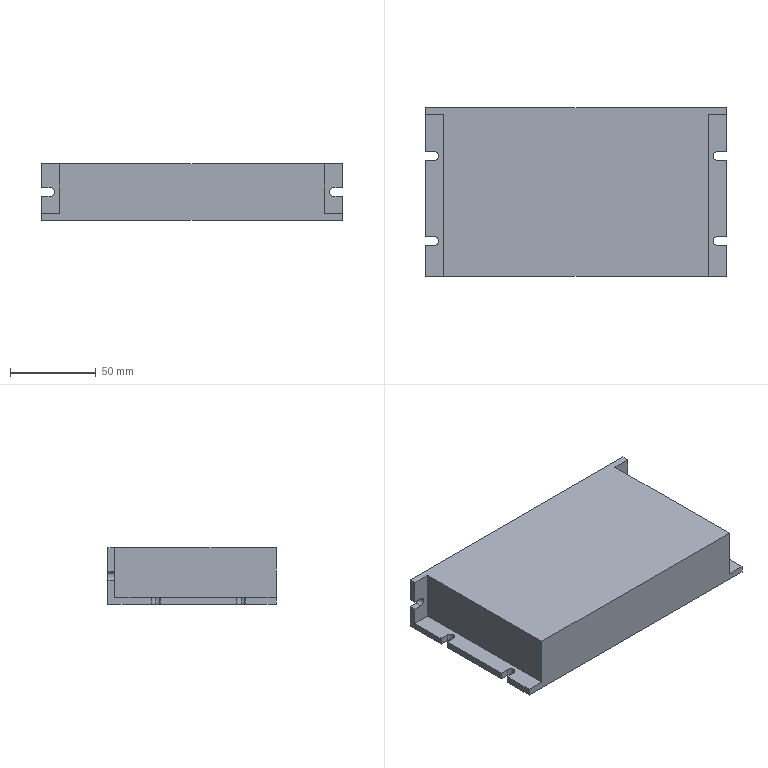Part | SolidWorks | features BaseBody 1 | 1 solid | 38 faces | box 175 x 98 x 33 mm | volume 507848 mm3 | plane 30 | cylinder 8 | commonest cylinder face diameters 5 x8
STEP:
#1=CARTESIAN_POINT('',(82.5,49.,14.));
#2=VERTEX_POINT('',#1);
#3=CARTESIAN_POINT('',(87.5,49.,14.));
#4=VERTEX_POINT('',#3);
#5=CARTESIAN_POINT('',(-87.5,49.,14.));
#6=DIRECTION('',(1.,0.,0.));
#7=VECTOR('',#6,1000.);
#8=LINE('',#5,#7);
#9=EDGE_CURVE('',#2,#4,#8,.T.);
#10=ORIENTED_EDGE('',*,*,#9,.F.);
#11=CARTESIAN_POINT('',(82.5,45.,14.));
#12=VERTEX_POINT('',#11);
#13=CARTESIAN_POINT('',(82.5,139.,14.));
#14=DIRECTION('',(0.,-1.,0.));
#15=VECTOR('',#14,1000.);
#16=LINE('',#13,#15);
#17=EDGE_CURVE('',#2,#12,#16,.T.);
#18=ORIENTED_EDGE('',*,*,#17,.T.);
#19=CARTESIAN_POINT('',(87.5,45.,14.));
#20=VERTEX_POINT('',#19);
#21=CARTESIAN_POINT('',(82.5,45.,14.));
#22=DIRECTION('',(1.,0.,0.));
#23=VECTOR('',#22,1000.);
#24=LINE('',#21,#23);
#25=EDGE_CURVE('',#12,#20,#24,.T.);
#26=ORIENTED_EDGE('',*,*,#25,.T.);
#27=CARTESIAN_POINT('',(87.5,-49.,14.));
#28=DIRECTION('',(0.,-1.,0.));
#29=VECTOR('',#28,1000.);
#30=LINE('',#27,#29);
#31=EDGE_CURVE('',#4,#20,#30,.T.);
#32=ORIENTED_EDGE('',*,*,#31,.F.);
#33=EDGE_LOOP('',(#10,#18,#26,#32));
#34=FACE_OUTER_BOUND('',#33,.T.);
#35=CARTESIAN_POINT('',(82.5,139.,14.));
#36=DIRECTION('',(0.,0.,-1.));
#37=DIRECTION('',(0.,-1.,0.));
#38=AXIS2_PLACEMENT_3D('',#35,#36,#37);
#39=PLANE('',#38);
#40=ADVANCED_FACE('',(#34),#39,.F.);
#41=CARTESIAN_POINT('',(82.5,45.,19.));
#42=VERTEX_POINT('',#41);
#43=CARTESIAN_POINT('',(87.5,45.,19.));
#44=VERTEX_POINT('',#43);
#45=CARTESIAN_POINT('',(0.,45.,19.));
#46=DIRECTION('',(1.,0.,0.));
#47=VECTOR('',#46,1000.);
#48=LINE('',#45,#47);
#49=EDGE_CURVE('',#42,#44,#48,.T.);
#50=ORIENTED_EDGE('',*,*,#49,.F.);
#51=CARTESIAN_POINT('',(82.5,49.,19.));
#52=VERTEX_POINT('',#51);
#53=CARTESIAN_POINT('',(82.5,139.,19.));
#54=DIRECTION('',(0.,-1.,0.));
#55=VECTOR('',#54,1000.);
#56=LINE('',#53,#55);
#57=EDGE_CURVE('',#52,#42,#56,.T.);
#58=ORIENTED_EDGE('',*,*,#57,.F.);
#59=CARTESIAN_POINT('',(87.5,49.,19.));
#60=VERTEX_POINT('',#59);
#61=CARTESIAN_POINT('',(-87.5,49.,19.));
#62=DIRECTION('',(-1.,0.,0.));
#63=VECTOR('',#62,1000.);
#64=LINE('',#61,#63);
#65=EDGE_CURVE('',#60,#52,#64,.T.);
#66=ORIENTED_EDGE('',*,*,#65,.F.);
#67=CARTESIAN_POINT('',(87.5,-49.,19.));
#68=DIRECTION('',(0.,1.,0.));
#69=VECTOR('',#68,1000.);
#70=LINE('',#67,#69);
#71=EDGE_CURVE('',#44,#60,#70,.T.);
#72=ORIENTED_EDGE('',*,*,#71,.F.);
#73=EDGE_LOOP('',(#50,#58,#66,#72));
#74=FACE_OUTER_BOUND('',#73,.T.);
#75=CARTESIAN_POINT('',(92.4,139.,19.));
#76=DIRECTION('',(0.,0.,1.));
#77=DIRECTION('',(1.,0.,0.));
#78=AXIS2_PLACEMENT_3D('',#75,#76,#77);
#79=PLANE('',#78);
#80=ADVANCED_FACE('',(#74),#79,.F.);
#81=ORIENTED_EDGE('',*,*,#57,.T.);
#82=CARTESIAN_POINT('',(82.5,45.,16.5));
#83=DIRECTION('',(0.,-1.,0.));
#84=DIRECTION('',(0.,0.,1.));
#85=AXIS2_PLACEMENT_3D('',#82,#83,#84);
#86=CIRCLE('',#85,2.5);
#87=EDGE_CURVE('',#42,#12,#86,.T.);
#88=ORIENTED_EDGE('',*,*,#87,.T.);
#89=ORIENTED_EDGE('',*,*,#17,.F.);
#90=CARTESIAN_POINT('',(82.5,49.,16.5));
#91=DIRECTION('',(0.,-1.,0.));
#92=DIRECTION('',(0.,0.,-1.));
#93=AXIS2_PLACEMENT_3D('',#90,#91,#92);
#94=CIRCLE('',#93,2.5);
#95=EDGE_CURVE('',#52,#2,#94,.T.);
#96=ORIENTED_EDGE('',*,*,#95,.F.);
#97=EDGE_LOOP('',(#81,#88,#89,#96));
#98=FACE_OUTER_BOUND('',#97,.T.);
#99=CARTESIAN_POINT('',(82.5,139.,16.5));
#100=DIRECTION('',(0.,-1.,0.));
#101=DIRECTION('',(0.,0.,-1.));
#102=AXIS2_PLACEMENT_3D('',#99,#100,#101);
#103=CYLINDRICAL_SURFACE('',#102,2.5);
#104=ADVANCED_FACE('',(#98),#103,.F.);
#105=CARTESIAN_POINT('',(-82.5,49.,19.));
#106=VERTEX_POINT('',#105);
#107=CARTESIAN_POINT('',(-82.5,45.,19.));
#108=VERTEX_POINT('',#107);
#109=CARTESIAN_POINT('',(-82.5,139.,19.));
#110=DIRECTION('',(0.,-1.,0.));
#111=VECTOR('',#110,1000.);
#112=LINE('',#109,#111);
#113=EDGE_CURVE('',#106,#108,#112,.T.);
#114=ORIENTED_EDGE('',*,*,#113,.T.);
#115=CARTESIAN_POINT('',(-87.5,45.,19.));
#116=VERTEX_POINT('',#115);
#117=CARTESIAN_POINT('',(-92.4,45.,19.));
#118=DIRECTION('',(-1.,0.,0.));
#119=VECTOR('',#118,1000.);
#120=LINE('',#117,#119);
#121=EDGE_CURVE('',#108,#116,#120,.T.);
#122=ORIENTED_EDGE('',*,*,#121,.T.);
#123=CARTESIAN_POINT('',(-87.5,49.,19.));
#124=VERTEX_POINT('',#123);
#125=CARTESIAN_POINT('',(-87.5,-49.,19.));
#126=DIRECTION('',(0.,-1.,0.));
#127=VECTOR('',#126,1000.);
#128=LINE('',#125,#127);
#129=EDGE_CURVE('',#124,#116,#128,.T.);
#130=ORIENTED_EDGE('',*,*,#129,.F.);
#131=CARTESIAN_POINT('',(-87.5,49.,19.));
#132=DIRECTION('',(-1.,0.,0.));
#133=VECTOR('',#132,1000.);
#134=LINE('',#131,#133);
#135=EDGE_CURVE('',#106,#124,#134,.T.);
#136=ORIENTED_EDGE('',*,*,#135,.F.);
#137=EDGE_LOOP('',(#114,#122,#130,#136));
#138=FACE_OUTER_BOUND('',#137,.T.);
#139=CARTESIAN_POINT('',(-92.4,139.,19.));
#140=DIRECTION('',(0.,0.,1.));
#141=DIRECTION('',(1.,0.,0.));
#142=AXIS2_PLACEMENT_3D('',#139,#140,#141);
#143=PLANE('',#142);
#144=ADVANCED_FACE('',(#138),#143,.F.);
#145=CARTESIAN_POINT('',(-87.5,45.,14.));
#146=VERTEX_POINT('',#145);
#147=CARTESIAN_POINT('',(-87.5,49.,14.));
#148=VERTEX_POINT('',#147);
#149=CARTESIAN_POINT('',(-87.5,-49.,14.));
#150=DIRECTION('',(0.,1.,0.));
#151=VECTOR('',#150,1000.);
#152=LINE('',#149,#151);
#153=EDGE_CURVE('',#146,#148,#152,.T.);
#154=ORIENTED_EDGE('',*,*,#153,.F.);
#155=CARTESIAN_POINT('',(-82.5,45.,14.));
#156=VERTEX_POINT('',#155);
#157=CARTESIAN_POINT('',(0.,45.,14.));
#158=DIRECTION('',(1.,0.,0.));
#159=VECTOR('',#158,1000.);
#160=LINE('',#157,#159);
#161=EDGE_CURVE('',#146,#156,#160,.T.);
#162=ORIENTED_EDGE('',*,*,#161,.T.);
#163=CARTESIAN_POINT('',(-82.5,49.,14.));
#164=VERTEX_POINT('',#163);
#165=CARTESIAN_POINT('',(-82.5,139.,14.));
#166=DIRECTION('',(0.,-1.,0.));
#167=VECTOR('',#166,1000.);
#168=LINE('',#165,#167);
#169=EDGE_CURVE('',#164,#156,#168,.T.);
#170=ORIENTED_EDGE('',*,*,#169,.F.);
#171=CARTESIAN_POINT('',(-87.5,49.,14.));
#172=DIRECTION('',(1.,0.,0.));
#173=VECTOR('',#172,1000.);
#174=LINE('',#171,#173);
#175=EDGE_CURVE('',#148,#164,#174,.T.);
#176=ORIENTED_EDGE('',*,*,#175,.F.);
#177=EDGE_LOOP('',(#154,#162,#170,#176));
#178=FACE_OUTER_BOUND('',#177,.T.);
#179=CARTESIAN_POINT('',(-82.5,139.,14.));
#180=DIRECTION('',(0.,0.,-1.));
#181=DIRECTION('',(0.,-1.,0.));
#182=AXIS2_PLACEMENT_3D('',#179,#180,#181);
#183=PLANE('',#182);
#184=ADVANCED_FACE('',(#178),#183,.F.);
#185=ORIENTED_EDGE('',*,*,#169,.T.);
#186=CARTESIAN_POINT('',(-82.5,45.,16.5));
#187=DIRECTION('',(0.,-1.,0.));
#188=DIRECTION('',(0.,0.,-1.));
#189=AXIS2_PLACEMENT_3D('',#186,#187,#188);
#190=CIRCLE('',#189,2.5);
#191=EDGE_CURVE('',#156,#108,#190,.T.);
#192=ORIENTED_EDGE('',*,*,#191,.T.);
#193=ORIENTED_EDGE('',*,*,#113,.F.);
#194=CARTESIAN_POINT('',(-82.5,49.,16.5));
#195=DIRECTION('',(0.,-1.,0.));
#196=DIRECTION('',(0.,0.,-1.));
#197=AXIS2_PLACEMENT_3D('',#194,#195,#196);
#198=CIRCLE('',#197,2.5);
#199=EDGE_CURVE('',#164,#106,#198,.T.);
#200=ORIENTED_EDGE('',*,*,#199,.F.);
#201=EDGE_LOOP('',(#185,#192,#193,#200));
#202=FACE_OUTER_BOUND('',#201,.T.);
#203=CARTESIAN_POINT('',(-82.5,139.,16.5));
#204=DIRECTION('',(0.,-1.,0.));
#205=DIRECTION('',(0.,0.,-1.));
#206=AXIS2_PLACEMENT_3D('',#203,#204,#205);
#207=CYLINDRICAL_SURFACE('',#206,2.5);
#208=ADVANCED_FACE('',(#202),#207,.F.);
#209=CARTESIAN_POINT('',(82.25,18.5,0.));
#210=VERTEX_POINT('',#209);
#211=CARTESIAN_POINT('',(82.25,23.5,0.));
#212=VERTEX_POINT('',#211);
#213=CARTESIAN_POINT('',(82.25,21.,0.));
#214=DIRECTION('',(0.,0.,-1.));
#215=DIRECTION('',(-1.,0.,0.));
#216=AXIS2_PLACEMENT_3D('',#213,#214,#215);
#217=CIRCLE('',#216,2.5);
#218=EDGE_CURVE('',#210,#212,#217,.T.);
#219=ORIENTED_EDGE('',*,*,#218,.T.);
#220=CARTESIAN_POINT('',(82.25,23.5,4.));
#221=VERTEX_POINT('',#220);
#222=CARTESIAN_POINT('',(82.25,23.5,-90.));
#223=DIRECTION('',(0.,0.,1.));
#224=VECTOR('',#223,1000.);
#225=LINE('',#222,#224);
#226=EDGE_CURVE('',#212,#221,#225,.T.);
#227=ORIENTED_EDGE('',*,*,#226,.T.);
#228=CARTESIAN_POINT('',(82.25,18.5,4.));
#229=VERTEX_POINT('',#228);
#230=CARTESIAN_POINT('',(82.25,21.,4.));
#231=DIRECTION('',(0.,0.,1.));
#232=DIRECTION('',(-1.,0.,0.));
#233=AXIS2_PLACEMENT_3D('',#230,#231,#232);
#234=CIRCLE('',#233,2.5);
#235=EDGE_CURVE('',#221,#229,#234,.T.);
#236=ORIENTED_EDGE('',*,*,#235,.T.);
#237=CARTESIAN_POINT('',(82.25,18.5,-90.));
#238=DIRECTION('',(0.,0.,1.));
#239=VECTOR('',#238,1000.);
#240=LINE('',#237,#239);
#241=EDGE_CURVE('',#210,#229,#240,.T.);
#242=ORIENTED_EDGE('',*,*,#241,.F.);
#243=EDGE_LOOP('',(#219,#227,#236,#242));
#244=FACE_OUTER_BOUND('',#243,.T.);
#245=CARTESIAN_POINT('',(82.25,21.,-90.));
#246=DIRECTION('',(0.,0.,1.));
#247=DIRECTION('',(1.,0.,0.));
#248=AXIS2_PLACEMENT_3D('',#245,#246,#247);
#249=CYLINDRICAL_SURFACE('',#248,2.5);
#250=ADVANCED_FACE('',(#244),#249,.F.);
#251=CARTESIAN_POINT('',(87.5,18.5,0.));
#252=VERTEX_POINT('',#251);
#253=CARTESIAN_POINT('',(0.,18.5,0.));
#254=DIRECTION('',(-1.,0.,0.));
#255=VECTOR('',#254,1000.);
#256=LINE('',#253,#255);
#257=EDGE_CURVE('',#252,#210,#256,.T.);
#258=ORIENTED_EDGE('',*,*,#257,.T.);
#259=ORIENTED_EDGE('',*,*,#241,.T.);
#260=CARTESIAN_POINT('',(87.5,18.5,4.));
#261=VERTEX_POINT('',#260);
#262=CARTESIAN_POINT('',(101.009,18.5,4.));
#263=DIRECTION('',(1.,0.,0.));
#264=VECTOR('',#263,1000.);
#265=LINE('',#262,#264);
#266=EDGE_CURVE('',#229,#261,#265,.T.);
#267=ORIENTED_EDGE('',*,*,#266,.T.);
#268=CARTESIAN_POINT('',(87.5,18.5,33.));
#269=DIRECTION('',(0.,0.,1.));
#270=VECTOR('',#269,1000.);
#271=LINE('',#268,#270);
#272=EDGE_CURVE('',#252,#261,#271,.T.);
#273=ORIENTED_EDGE('',*,*,#272,.F.);
#274=EDGE_LOOP('',(#258,#259,#267,#273));
#275=FACE_OUTER_BOUND('',#274,.T.);
#276=CARTESIAN_POINT('',(101.009,18.5,-90.));
#277=DIRECTION('',(0.,-1.,0.));
#278=DIRECTION('',(0.,0.,-1.));
#279=AXIS2_PLACEMENT_3D('',#276,#277,#278);
#280=PLANE('',#279);
#281=ADVANCED_FACE('',(#275),#280,.F.);
#282=CARTESIAN_POINT('',(87.5,23.5,4.));
#283=VERTEX_POINT('',#282);
#284=CARTESIAN_POINT('',(87.5,23.5,4.));
#285=DIRECTION('',(1.,0.,0.));
#286=VECTOR('',#285,1000.);
#287=LINE('',#284,#286);
#288=EDGE_CURVE('',#221,#283,#287,.T.);
#289=ORIENTED_EDGE('',*,*,#288,.F.);
#290=ORIENTED_EDGE('',*,*,#226,.F.);
#291=CARTESIAN_POINT('',(87.5,23.5,0.));
#292=VERTEX_POINT('',#291);
#293=CARTESIAN_POINT('',(0.,23.5,0.));
#294=DIRECTION('',(1.,0.,0.));
#295=VECTOR('',#294,1000.);
#296=LINE('',#293,#295);
#297=EDGE_CURVE('',#212,#292,#296,.T.);
#298=ORIENTED_EDGE('',*,*,#297,.T.);
#299=CARTESIAN_POINT('',(87.5,23.5,33.));
#300=DIRECTION('',(0.,0.,-1.));
#301=VECTOR('',#300,1000.);
#302=LINE('',#299,#301);
#303=EDGE_CURVE('',#283,#292,#302,.T.);
#304=ORIENTED_EDGE('',*,*,#303,.F.);
#305=EDGE_LOOP('',(#289,#290,#298,#304));
#306=FACE_OUTER_BOUND('',#305,.T.);
#307=CARTESIAN_POINT('',(82.25,23.5,-90.));
#308=DIRECTION('',(0.,1.,0.));
#309=DIRECTION('',(1.,0.,0.));
#310=AXIS2_PLACEMENT_3D('',#307,#308,#309);
#311=PLANE('',#310);
#312=ADVANCED_FACE('',(#306),#311,.F.);
#313=CARTESIAN_POINT('',(82.25,-31.,0.));
#314=VERTEX_POINT('',#313);
#315=CARTESIAN_POINT('',(82.25,-26.,0.));
#316=VERTEX_POINT('',#315);
#317=CARTESIAN_POINT('',(82.25,-28.5,0.));
#318=DIRECTION('',(0.,0.,-1.));
#319=DIRECTION('',(-1.,0.,0.));
#320=AXIS2_PLACEMENT_3D('',#317,#318,#319);
#321=CIRCLE('',#320,2.5);
#322=EDGE_CURVE('',#314,#316,#321,.T.);
#323=ORIENTED_EDGE('',*,*,#322,.T.);
#324=CARTESIAN_POINT('',(82.25,-26.,4.));
#325=VERTEX_POINT('',#324);
#326=CARTESIAN_POINT('',(82.25,-26.,-90.));
#327=DIRECTION('',(0.,0.,1.));
#328=VECTOR('',#327,1000.);
#329=LINE('',#326,#328);
#330=EDGE_CURVE('',#316,#325,#329,.T.);
#331=ORIENTED_EDGE('',*,*,#330,.T.);
#332=CARTESIAN_POINT('',(82.25,-31.,4.));
#333=VERTEX_POINT('',#332);
#334=CARTESIAN_POINT('',(82.25,-28.5,4.));
#335=DIRECTION('',(0.,0.,1.));
#336=DIRECTION('',(-1.,0.,0.));
#337=AXIS2_PLACEMENT_3D('',#334,#335,#336);
#338=CIRCLE('',#337,2.5);
#339=EDGE_CURVE('',#325,#333,#338,.T.);
#340=ORIENTED_EDGE('',*,*,#339,.T.);
#341=CARTESIAN_POINT('',(82.25,-31.,-90.));
#342=DIRECTION('',(0.,0.,1.));
#343=VECTOR('',#342,1000.);
#344=LINE('',#341,#343);
#345=EDGE_CURVE('',#314,#333,#344,.T.);
#346=ORIENTED_EDGE('',*,*,#345,.F.);
#347=EDGE_LOOP('',(#323,#331,#340,#346));
#348=FACE_OUTER_BOUND('',#347,.T.);
#349=CARTESIAN_POINT('',(82.25,-28.5,-90.));
#350=DIRECTION('',(0.,0.,1.));
#351=DIRECTION('',(1.,0.,0.));
#352=AXIS2_PLACEMENT_3D('',#349,#350,#351);
#353=CYLINDRICAL_SURFACE('',#352,2.5);
#354=ADVANCED_FACE('',(#348),#353,.F.);
#355=CARTESIAN_POINT('',(87.5,-31.,0.));
#356=VERTEX_POINT('',#355);
#357=CARTESIAN_POINT('',(0.,-31.,0.));
#358=DIRECTION('',(-1.,0.,0.));
#359=VECTOR('',#358,1000.);
#360=LINE('',#357,#359);
#361=EDGE_CURVE('',#356,#314,#360,.T.);
#362=ORIENTED_EDGE('',*,*,#361,.T.);
#363=ORIENTED_EDGE('',*,*,#345,.T.);
#364=CARTESIAN_POINT('',(87.5,-31.,4.));
#365=VERTEX_POINT('',#364);
#366=CARTESIAN_POINT('',(82.25,-31.,4.));
#367=DIRECTION('',(1.,0.,0.));
#368=VECTOR('',#367,1000.);
#369=LINE('',#366,#368);
#370=EDGE_CURVE('',#333,#365,#369,.T.);
#371=ORIENTED_EDGE('',*,*,#370,.T.);
#372=CARTESIAN_POINT('',(87.5,-31.,33.));
#373=DIRECTION('',(0.,0.,1.));
#374=VECTOR('',#373,1000.);
#375=LINE('',#372,#374);
#376=EDGE_CURVE('',#356,#365,#375,.T.);
#377=ORIENTED_EDGE('',*,*,#376,.F.);
#378=EDGE_LOOP('',(#362,#363,#371,#377));
#379=FACE_OUTER_BOUND('',#378,.T.);
#380=CARTESIAN_POINT('',(82.25,-31.,-90.));
#381=DIRECTION('',(0.,-1.,0.));
#382=DIRECTION('',(0.,0.,-1.));
#383=AXIS2_PLACEMENT_3D('',#380,#381,#382);
#384=PLANE('',#383);
#385=ADVANCED_FACE('',(#379),#384,.F.);
#386=CARTESIAN_POINT('',(87.5,-26.,4.));
#387=VERTEX_POINT('',#386);
#388=CARTESIAN_POINT('',(87.5,-26.,4.));
#389=DIRECTION('',(1.,0.,0.));
#390=VECTOR('',#389,1000.);
#391=LINE('',#388,#390);
#392=EDGE_CURVE('',#325,#387,#391,.T.);
#393=ORIENTED_EDGE('',*,*,#392,.F.);
#394=ORIENTED_EDGE('',*,*,#330,.F.);
#395=CARTESIAN_POINT('',(87.5,-26.,0.));
#396=VERTEX_POINT('',#395);
#397=CARTESIAN_POINT('',(0.,-26.,0.));
#398=DIRECTION('',(1.,0.,0.));
#399=VECTOR('',#398,1000.);
#400=LINE('',#397,#399);
#401=EDGE_CURVE('',#316,#396,#400,.T.);
#402=ORIENTED_EDGE('',*,*,#401,.T.);
#403=CARTESIAN_POINT('',(87.5,-26.,33.));
#404=DIRECTION('',(0.,0.,-1.));
#405=VECTOR('',#404,1000.);
#406=LINE('',#403,#405);
#407=EDGE_CURVE('',#387,#396,#406,.T.);
#408=ORIENTED_EDGE('',*,*,#407,.F.);
#409=EDGE_LOOP('',(#393,#394,#402,#408));
#410=FACE_OUTER_BOUND('',#409,.T.);
#411=CARTESIAN_POINT('',(101.009,-26.,-90.));
#412=DIRECTION('',(0.,1.,0.));
#413=DIRECTION('',(1.,0.,0.));
#414=AXIS2_PLACEMENT_3D('',#411,#412,#413);
#415=PLANE('',#414);
#416=ADVANCED_FACE('',(#410),#415,.F.);
#417=CARTESIAN_POINT('',(-79.75,-28.5,0.));
#418=VERTEX_POINT('',#417);
#419=CARTESIAN_POINT('',(-79.75,-28.5,4.));
#420=VERTEX_POINT('',#419);
#421=CARTESIAN_POINT('',(-79.75,-28.5,-90.));
#422=DIRECTION('',(0.,0.,1.));
#423=VECTOR('',#422,1000.);
#424=LINE('',#421,#423);
#425=EDGE_CURVE('',#418,#420,#424,.T.);
#426=ORIENTED_EDGE('',*,*,#425,.F.);
#427=CARTESIAN_POINT('',(-82.25,-31.,0.));
#428=VERTEX_POINT('',#427);
#429=CARTESIAN_POINT('',(-82.25,-28.5,0.));
#430=DIRECTION('',(0.,0.,-1.));
#431=DIRECTION('',(-1.,0.,0.));
#432=AXIS2_PLACEMENT_3D('',#429,#430,#431);
#433=CIRCLE('',#432,2.5);
#434=EDGE_CURVE('',#418,#428,#433,.T.);
#435=ORIENTED_EDGE('',*,*,#434,.T.);
#436=CARTESIAN_POINT('',(-82.25,-31.,4.));
#437=VERTEX_POINT('',#436);
#438=CARTESIAN_POINT('',(-82.25,-31.,-90.));
#439=DIRECTION('',(0.,0.,1.));
#440=VECTOR('',#439,1000.);
#441=LINE('',#438,#440);
#442=EDGE_CURVE('',#428,#437,#441,.T.);
#443=ORIENTED_EDGE('',*,*,#442,.T.);
#444=CARTESIAN_POINT('',(-82.25,-28.5,4.));
#445=DIRECTION('',(0.,0.,1.));
#446=DIRECTION('',(1.,0.,0.));
#447=AXIS2_PLACEMENT_3D('',#444,#445,#446);
#448=CIRCLE('',#447,2.5);
#449=EDGE_CURVE('',#437,#420,#448,.T.);
#450=ORIENTED_EDGE('',*,*,#449,.T.);
#451=EDGE_LOOP('',(#426,#435,#443,#450));
#452=FACE_OUTER_BOUND('',#451,.T.);
#453=CARTESIAN_POINT('',(-82.25,-28.5,-90.));
#454=DIRECTION('',(0.,0.,1.));
#455=DIRECTION('',(1.,0.,0.));
#456=AXIS2_PLACEMENT_3D('',#453,#454,#455);
#457=CYLINDRICAL_SURFACE('',#456,2.5);
#458=ADVANCED_FACE('',(#452),#457,.F.);
#459=CARTESIAN_POINT('',(-87.5,-26.,0.));
#460=VERTEX_POINT('',#459);
#461=CARTESIAN_POINT('',(-82.25,-26.,0.));
#462=VERTEX_POINT('',#461);
#463=CARTESIAN_POINT('',(0.,-26.,0.));
#464=DIRECTION('',(1.,0.,0.));
#465=VECTOR('',#464,1000.);
#466=LINE('',#463,#465);
#467=EDGE_CURVE('',#460,#462,#466,.T.);
#468=ORIENTED_EDGE('',*,*,#467,.T.);
#469=CARTESIAN_POINT('',(-82.25,-26.,4.));
#470=VERTEX_POINT('',#469);
#471=CARTESIAN_POINT('',(-82.25,-26.,-90.));
#472=DIRECTION('',(0.,0.,1.));
#473=VECTOR('',#472,1000.);
#474=LINE('',#471,#473);
#475=EDGE_CURVE('',#462,#470,#474,.T.);
#476=ORIENTED_EDGE('',*,*,#475,.T.);
#477=CARTESIAN_POINT('',(-87.5,-26.,4.));
#478=VERTEX_POINT('',#477);
#479=CARTESIAN_POINT('',(-101.009,-26.,4.));
#480=DIRECTION('',(-1.,0.,0.));
#481=VECTOR('',#480,1000.);
#482=LINE('',#479,#481);
#483=EDGE_CURVE('',#470,#478,#482,.T.);
#484=ORIENTED_EDGE('',*,*,#483,.T.);
#485=CARTESIAN_POINT('',(-87.5,-26.,33.));
#486=DIRECTION('',(0.,0.,1.));
#487=VECTOR('',#486,1000.);
#488=LINE('',#485,#487);
#489=EDGE_CURVE('',#460,#478,#488,.T.);
#490=ORIENTED_EDGE('',*,*,#489,.F.);
#491=EDGE_LOOP('',(#468,#476,#484,#490));
#492=FACE_OUTER_BOUND('',#491,.T.);
#493=CARTESIAN_POINT('',(-101.009,-26.,-90.));
#494=DIRECTION('',(0.,1.,0.));
#495=DIRECTION('',(1.,0.,0.));
#496=AXIS2_PLACEMENT_3D('',#493,#494,#495);
#497=PLANE('',#496);
#498=ADVANCED_FACE('',(#492),#497,.F.);
#499=CARTESIAN_POINT('',(-87.5,-31.,4.));
#500=VERTEX_POINT('',#499);
#501=CARTESIAN_POINT('',(-87.5,-31.,4.));
#502=DIRECTION('',(-1.,0.,0.));
#503=VECTOR('',#502,1000.);
#504=LINE('',#501,#503);
#505=EDGE_CURVE('',#437,#500,#504,.T.);
#506=ORIENTED_EDGE('',*,*,#505,.F.);
#507=ORIENTED_EDGE('',*,*,#442,.F.);
#508=CARTESIAN_POINT('',(-87.5,-31.,0.));
#509=VERTEX_POINT('',#508);
#510=CARTESIAN_POINT('',(0.,-31.,0.));
#511=DIRECTION('',(-1.,0.,0.));
#512=VECTOR('',#511,1000.);
#513=LINE('',#510,#512);
#514=EDGE_CURVE('',#428,#509,#513,.T.);
#515=ORIENTED_EDGE('',*,*,#514,.T.);
#516=CARTESIAN_POINT('',(-87.5,-31.,33.));
#517=DIRECTION('',(0.,0.,-1.));
#518=VECTOR('',#517,1000.);
#519=LINE('',#516,#518);
#520=EDGE_CURVE('',#500,#509,#519,.T.);
#521=ORIENTED_EDGE('',*,*,#520,.F.);
#522=EDGE_LOOP('',(#506,#507,#515,#521));
#523=FACE_OUTER_BOUND('',#522,.T.);
#524=CARTESIAN_POINT('',(-82.25,-31.,-90.));
#525=DIRECTION('',(0.,-1.,0.));
#526=DIRECTION('',(0.,0.,-1.));
#527=AXIS2_PLACEMENT_3D('',#524,#525,#526);
#528=PLANE('',#527);
#529=ADVANCED_FACE('',(#523),#528,.F.);
#530=CARTESIAN_POINT('',(-79.75,21.,0.));
#531=VERTEX_POINT('',#530);
#532=CARTESIAN_POINT('',(-79.75,21.,4.));
#533=VERTEX_POINT('',#532);
#534=CARTESIAN_POINT('',(-79.75,21.,-90.));
#535=DIRECTION('',(0.,0.,1.));
#536=VECTOR('',#535,1000.);
#537=LINE('',#534,#536);
#538=EDGE_CURVE('',#531,#533,#537,.T.);
#539=ORIENTED_EDGE('',*,*,#538,.F.);
#540=CARTESIAN_POINT('',(-82.25,18.5,0.));
#541=VERTEX_POINT('',#540);
#542=CARTESIAN_POINT('',(-82.25,21.,0.));
#543=DIRECTION('',(0.,0.,-1.));
#544=DIRECTION('',(-1.,0.,0.));
#545=AXIS2_PLACEMENT_3D('',#542,#543,#544);
#546=CIRCLE('',#545,2.5);
#547=EDGE_CURVE('',#531,#541,#546,.T.);
#548=ORIENTED_EDGE('',*,*,#547,.T.);
#549=CARTESIAN_POINT('',(-82.25,18.5,4.));
#550=VERTEX_POINT('',#549);
#551=CARTESIAN_POINT('',(-82.25,18.5,-90.));
#552=DIRECTION('',(0.,0.,1.));
#553=VECTOR('',#552,1000.);
#554=LINE('',#551,#553);
#555=EDGE_CURVE('',#541,#550,#554,.T.);
#556=ORIENTED_EDGE('',*,*,#555,.T.);
#557=CARTESIAN_POINT('',(-82.25,21.,4.));
#558=DIRECTION('',(0.,0.,1.));
#559=DIRECTION('',(1.,0.,0.));
#560=AXIS2_PLACEMENT_3D('',#557,#558,#559);
#561=CIRCLE('',#560,2.5);
#562=EDGE_CURVE('',#550,#533,#561,.T.);
#563=ORIENTED_EDGE('',*,*,#562,.T.);
#564=EDGE_LOOP('',(#539,#548,#556,#563));
#565=FACE_OUTER_BOUND('',#564,.T.);
#566=CARTESIAN_POINT('',(-82.25,21.,-90.));
#567=DIRECTION('',(0.,0.,1.));
#568=DIRECTION('',(1.,0.,0.));
#569=AXIS2_PLACEMENT_3D('',#566,#567,#568);
#570=CYLINDRICAL_SURFACE('',#569,2.5);
#571=ADVANCED_FACE('',(#565),#570,.F.);
#572=CARTESIAN_POINT('',(-87.5,23.5,0.));
#573=VERTEX_POINT('',#572);
#574=CARTESIAN_POINT('',(-82.25,23.5,0.));
#575=VERTEX_POINT('',#574);
#576=CARTESIAN_POINT('',(0.,23.5,0.));
#577=DIRECTION('',(1.,0.,0.));
#578=VECTOR('',#577,1000.);
#579=LINE('',#576,#578);
#580=EDGE_CURVE('',#573,#575,#579,.T.);
#581=ORIENTED_EDGE('',*,*,#580,.T.);
#582=CARTESIAN_POINT('',(-82.25,23.5,4.));
#583=VERTEX_POINT('',#582);
#584=CARTESIAN_POINT('',(-82.25,23.5,-90.));
#585=DIRECTION('',(0.,0.,1.));
#586=VECTOR('',#585,1000.);
#587=LINE('',#584,#586);
#588=EDGE_CURVE('',#575,#583,#587,.T.);
#589=ORIENTED_EDGE('',*,*,#588,.T.);
#590=CARTESIAN_POINT('',(-87.5,23.5,4.));
#591=VERTEX_POINT('',#590);
#592=CARTESIAN_POINT('',(-82.25,23.5,4.));
#593=DIRECTION('',(-1.,0.,0.));
#594=VECTOR('',#593,1000.);
#595=LINE('',#592,#594);
#596=EDGE_CURVE('',#583,#591,#595,.T.);
#597=ORIENTED_EDGE('',*,*,#596,.T.);
#598=CARTESIAN_POINT('',(-87.5,23.5,33.));
#599=DIRECTION('',(0.,0.,1.));
#600=VECTOR('',#599,1000.);
#601=LINE('',#598,#600);
#602=EDGE_CURVE('',#573,#591,#601,.T.);
#603=ORIENTED_EDGE('',*,*,#602,.F.);
#604=EDGE_LOOP('',(#581,#589,#597,#603));
#605=FACE_OUTER_BOUND('',#604,.T.);
#606=CARTESIAN_POINT('',(-82.25,23.5,-90.));
#607=DIRECTION('',(0.,1.,0.));
#608=DIRECTION('',(1.,0.,0.));
#609=AXIS2_PLACEMENT_3D('',#606,#607,#608);
#610=PLANE('',#609);
#611=ADVANCED_FACE('',(#605),#610,.F.);
#612=CARTESIAN_POINT('',(-87.5,18.5,4.));
#613=VERTEX_POINT('',#612);
#614=CARTESIAN_POINT('',(-87.5,18.5,4.));
#615=DIRECTION('',(-1.,0.,0.));
#616=VECTOR('',#615,1000.);
#617=LINE('',#614,#616);
#618=EDGE_CURVE('',#550,#613,#617,.T.);
#619=ORIENTED_EDGE('',*,*,#618,.F.);
#620=ORIENTED_EDGE('',*,*,#555,.F.);
#621=CARTESIAN_POINT('',(-87.5,18.5,0.));
#622=VERTEX_POINT('',#621);
#623=CARTESIAN_POINT('',(0.,18.5,0.));
#624=DIRECTION('',(-1.,0.,0.));
#625=VECTOR('',#624,1000.);
#626=LINE('',#623,#625);
#627=EDGE_CURVE('',#541,#622,#626,.T.);
#628=ORIENTED_EDGE('',*,*,#627,.T.);
#629=CARTESIAN_POINT('',(-87.5,18.5,33.));
#630=DIRECTION('',(0.,0.,-1.));
#631=VECTOR('',#630,1000.);
#632=LINE('',#629,#631);
#633=EDGE_CURVE('',#613,#622,#632,.T.);
#634=ORIENTED_EDGE('',*,*,#633,.F.);
#635=EDGE_LOOP('',(#619,#620,#628,#634));
#636=FACE_OUTER_BOUND('',#635,.T.);
#637=CARTESIAN_POINT('',(-101.009,18.5,-90.));
#638=DIRECTION('',(0.,-1.,0.));
#639=DIRECTION('',(0.,0.,-1.));
#640=AXIS2_PLACEMENT_3D('',#637,#638,#639);
#641=PLANE('',#640);
#642=ADVANCED_FACE('',(#636),#641,.F.);
#643=ORIENTED_EDGE('',*,*,#161,.F.);
#644=CARTESIAN_POINT('',(-87.5,45.,4.));
#645=VERTEX_POINT('',#644);
#646=CARTESIAN_POINT('',(-87.5,45.,33.));
#647=DIRECTION('',(0.,0.,-1.));
#648=VECTOR('',#647,1000.);
#649=LINE('',#646,#648);
#650=EDGE_CURVE('',#146,#645,#649,.T.);
#651=ORIENTED_EDGE('',*,*,#650,.T.);
#652=CARTESIAN_POINT('',(-77.,45.,4.));
#653=VERTEX_POINT('',#652);
#654=CARTESIAN_POINT('',(-87.5,45.,4.));
#655=DIRECTION('',(1.,0.,0.));
#656=VECTOR('',#655,1000.);
#657=LINE('',#654,#656);
#658=EDGE_CURVE('',#645,#653,#657,.T.);
#659=ORIENTED_EDGE('',*,*,#658,.T.);
#660=CARTESIAN_POINT('',(-77.,45.,33.));
#661=VERTEX_POINT('',#660);
#662=CARTESIAN_POINT('',(-77.,45.,33.));
#663=DIRECTION('',(0.,0.,1.));
#664=VECTOR('',#663,1000.);
#665=LINE('',#662,#664);
#666=EDGE_CURVE('',#653,#661,#665,.T.);
#667=ORIENTED_EDGE('',*,*,#666,.T.);
#668=CARTESIAN_POINT('',(-87.5,45.,33.));
#669=VERTEX_POINT('',#668);
#670=CARTESIAN_POINT('',(-87.5,45.,33.));
#671=DIRECTION('',(-1.,0.,0.));
#672=VECTOR('',#671,1000.);
#673=LINE('',#670,#672);
#674=EDGE_CURVE('',#661,#669,#673,.T.);
#675=ORIENTED_EDGE('',*,*,#674,.T.);
#676=CARTESIAN_POINT('',(-87.5,45.,33.));
#677=DIRECTION('',(0.,0.,-1.));
#678=VECTOR('',#677,1000.);
#679=LINE('',#676,#678);
#680=EDGE_CURVE('',#669,#116,#679,.T.);
#681=ORIENTED_EDGE('',*,*,#680,.T.);
#682=ORIENTED_EDGE('',*,*,#121,.F.);
#683=ORIENTED_EDGE('',*,*,#191,.F.);
#684=EDGE_LOOP('',(#643,#651,#659,#667,#675,#681,#682,#683));
#685=FACE_OUTER_BOUND('',#684,.T.);
#686=CARTESIAN_POINT('',(0.,45.,0.));
#687=DIRECTION('',(0.,-1.,0.));
#688=DIRECTION('',(0.,0.,-1.));
#689=AXIS2_PLACEMENT_3D('',#686,#687,#688);
#690=PLANE('',#689);
#691=ADVANCED_FACE('',(#685),#690,.T.);
#692=ORIENTED_EDGE('',*,*,#449,.F.);
#693=ORIENTED_EDGE('',*,*,#505,.T.);
#694=CARTESIAN_POINT('',(-87.5,-49.,4.));
#695=VERTEX_POINT('',#694);
#696=CARTESIAN_POINT('',(-87.5,45.,4.));
#697=DIRECTION('',(0.,-1.,0.));
#698=VECTOR('',#697,1000.);
#699=LINE('',#696,#698);
#700=EDGE_CURVE('',#500,#695,#699,.T.);
#701=ORIENTED_EDGE('',*,*,#700,.T.);
#702=CARTESIAN_POINT('',(-77.,-49.,4.));
#703=VERTEX_POINT('',#702);
#704=CARTESIAN_POINT('',(-87.5,-49.,4.));
#705=DIRECTION('',(1.,0.,0.));
#706=VECTOR('',#705,1000.);
#707=LINE('',#704,#706);
#708=EDGE_CURVE('',#695,#703,#707,.T.);
#709=ORIENTED_EDGE('',*,*,#708,.T.);
#710=CARTESIAN_POINT('',(-77.,45.,4.));
#711=DIRECTION('',(0.,-1.,0.));
#712=VECTOR('',#711,1000.);
#713=LINE('',#710,#712);
#714=EDGE_CURVE('',#653,#703,#713,.T.);
#715=ORIENTED_EDGE('',*,*,#714,.F.);
#716=ORIENTED_EDGE('',*,*,#658,.F.);
#717=CARTESIAN_POINT('',(-87.5,45.,4.));
#718=DIRECTION('',(0.,-1.,0.));
#719=VECTOR('',#718,1000.);
#720=LINE('',#717,#719);
#721=EDGE_CURVE('',#645,#591,#720,.T.);
#722=ORIENTED_EDGE('',*,*,#721,.T.);
#723=ORIENTED_EDGE('',*,*,#596,.F.);
#724=CARTESIAN_POINT('',(-82.25,21.,4.));
#725=DIRECTION('',(0.,0.,1.));
#726=DIRECTION('',(1.,0.,0.));
#727=AXIS2_PLACEMENT_3D('',#724,#725,#726);
#728=CIRCLE('',#727,2.5);
#729=EDGE_CURVE('',#533,#583,#728,.T.);
#730=ORIENTED_EDGE('',*,*,#729,.F.);
#731=ORIENTED_EDGE('',*,*,#562,.F.);
#732=ORIENTED_EDGE('',*,*,#618,.T.);
#733=CARTESIAN_POINT('',(-87.5,45.,4.));
#734=DIRECTION('',(0.,-1.,0.));
#735=VECTOR('',#734,1000.);
#736=LINE('',#733,#735);
#737=EDGE_CURVE('',#613,#478,#736,.T.);
#738=ORIENTED_EDGE('',*,*,#737,.T.);
#739=ORIENTED_EDGE('',*,*,#483,.F.);
#740=CARTESIAN_POINT('',(-82.25,-28.5,4.));
#741=DIRECTION('',(0.,0.,1.));
#742=DIRECTION('',(1.,0.,0.));
#743=AXIS2_PLACEMENT_3D('',#740,#741,#742);
#744=CIRCLE('',#743,2.5);
#745=EDGE_CURVE('',#420,#470,#744,.T.);
#746=ORIENTED_EDGE('',*,*,#745,.F.);
#747=EDGE_LOOP('',(#692,#693,#701,#709,#715,#716,#722,#723,#730,#731,#732,#738,#739,#746));
#748=FACE_OUTER_BOUND('',#747,.T.);
#749=CARTESIAN_POINT('',(-87.5,45.,4.));
#750=DIRECTION('',(0.,0.,-1.));
#751=DIRECTION('',(0.,-1.,0.));
#752=AXIS2_PLACEMENT_3D('',#749,#750,#751);
#753=PLANE('',#752);
#754=ADVANCED_FACE('',(#748),#753,.F.);
#755=CARTESIAN_POINT('',(-77.,-49.,33.));
#756=VERTEX_POINT('',#755);
#757=CARTESIAN_POINT('',(-77.,-49.,33.));
#758=DIRECTION('',(0.,0.,1.));
#759=VECTOR('',#758,1000.);
#760=LINE('',#757,#759);
#761=EDGE_CURVE('',#703,#756,#760,.T.);
#762=ORIENTED_EDGE('',*,*,#761,.T.);
#763=CARTESIAN_POINT('',(-77.,45.,33.));
#764=DIRECTION('',(0.,-1.,0.));
#765=VECTOR('',#764,1000.);
#766=LINE('',#763,#765);
#767=EDGE_CURVE('',#661,#756,#766,.T.);
#768=ORIENTED_EDGE('',*,*,#767,.F.);
#769=ORIENTED_EDGE('',*,*,#666,.F.);
#770=ORIENTED_EDGE('',*,*,#714,.T.);
#771=EDGE_LOOP('',(#762,#768,#769,#770));
#772=FACE_OUTER_BOUND('',#771,.T.);
#773=CARTESIAN_POINT('',(-77.,45.,33.));
#774=DIRECTION('',(1.,0.,0.));
#775=DIRECTION('',(0.,1.,0.));
#776=AXIS2_PLACEMENT_3D('',#773,#774,#775);
#777=PLANE('',#776);
#778=ADVANCED_FACE('',(#772),#777,.F.);
#779=ORIENTED_EDGE('',*,*,#87,.F.);
#780=ORIENTED_EDGE('',*,*,#49,.T.);
#781=CARTESIAN_POINT('',(87.5,45.,33.));
#782=VERTEX_POINT('',#781);
#783=CARTESIAN_POINT('',(87.5,45.,33.));
#784=DIRECTION('',(0.,0.,1.));
#785=VECTOR('',#784,1000.);
#786=LINE('',#783,#785);
#787=EDGE_CURVE('',#44,#782,#786,.T.);
#788=ORIENTED_EDGE('',*,*,#787,.T.);
#789=CARTESIAN_POINT('',(77.,45.,33.));
#790=VERTEX_POINT('',#789);
#791=CARTESIAN_POINT('',(87.5,45.,33.));
#792=DIRECTION('',(-1.,0.,0.));
#793=VECTOR('',#792,1000.);
#794=LINE('',#791,#793);
#795=EDGE_CURVE('',#782,#790,#794,.T.);
#796=ORIENTED_EDGE('',*,*,#795,.T.);
#797=CARTESIAN_POINT('',(77.,45.,4.));
#798=VERTEX_POINT('',#797);
#799=CARTESIAN_POINT('',(77.,45.,33.));
#800=DIRECTION('',(0.,0.,-1.));
#801=VECTOR('',#800,1000.);
#802=LINE('',#799,#801);
#803=EDGE_CURVE('',#790,#798,#802,.T.);
#804=ORIENTED_EDGE('',*,*,#803,.T.);
#805=CARTESIAN_POINT('',(87.5,45.,4.));
#806=VERTEX_POINT('',#805);
#807=CARTESIAN_POINT('',(87.5,45.,4.));
#808=DIRECTION('',(1.,0.,0.));
#809=VECTOR('',#808,1000.);
#810=LINE('',#807,#809);
#811=EDGE_CURVE('',#798,#806,#810,.T.);
#812=ORIENTED_EDGE('',*,*,#811,.T.);
#813=CARTESIAN_POINT('',(87.5,45.,33.));
#814=DIRECTION('',(0.,0.,1.));
#815=VECTOR('',#814,1000.);
#816=LINE('',#813,#815);
#817=EDGE_CURVE('',#806,#20,#816,.T.);
#818=ORIENTED_EDGE('',*,*,#817,.T.);
#819=ORIENTED_EDGE('',*,*,#25,.F.);
#820=EDGE_LOOP('',(#779,#780,#788,#796,#804,#812,#818,#819));
#821=FACE_OUTER_BOUND('',#820,.T.);
#822=CARTESIAN_POINT('',(0.,45.,0.));
#823=DIRECTION('',(0.,1.,0.));
#824=DIRECTION('',(1.,0.,0.));
#825=AXIS2_PLACEMENT_3D('',#822,#823,#824);
#826=PLANE('',#825);
#827=ADVANCED_FACE('',(#821),#826,.F.);
#828=CARTESIAN_POINT('',(77.,-49.,33.));
#829=VERTEX_POINT('',#828);
#830=CARTESIAN_POINT('',(77.,-49.,4.));
#831=VERTEX_POINT('',#830);
#832=CARTESIAN_POINT('',(77.,-49.,33.));
#833=DIRECTION('',(0.,0.,-1.));
#834=VECTOR('',#833,1000.);
#835=LINE('',#832,#834);
#836=EDGE_CURVE('',#829,#831,#835,.T.);
#837=ORIENTED_EDGE('',*,*,#836,.T.);
#838=CARTESIAN_POINT('',(77.,45.,4.));
#839=DIRECTION('',(0.,-1.,0.));
#840=VECTOR('',#839,1000.);
#841=LINE('',#838,#840);
#842=EDGE_CURVE('',#798,#831,#841,.T.);
#843=ORIENTED_EDGE('',*,*,#842,.F.);
#844=ORIENTED_EDGE('',*,*,#803,.F.);
#845=CARTESIAN_POINT('',(77.,45.,33.));
#846=DIRECTION('',(0.,-1.,0.));
#847=VECTOR('',#846,1000.);
#848=LINE('',#845,#847);
#849=EDGE_CURVE('',#790,#829,#848,.T.);
#850=ORIENTED_EDGE('',*,*,#849,.T.);
#851=EDGE_LOOP('',(#837,#843,#844,#850));
#852=FACE_OUTER_BOUND('',#851,.T.);
#853=CARTESIAN_POINT('',(77.,45.,33.));
#854=DIRECTION('',(-1.,0.,0.));
#855=DIRECTION('',(0.,0.,1.));
#856=AXIS2_PLACEMENT_3D('',#853,#854,#855);
#857=PLANE('',#856);
#858=ADVANCED_FACE('',(#852),#857,.F.);
#859=ORIENTED_EDGE('',*,*,#235,.F.);
#860=ORIENTED_EDGE('',*,*,#288,.T.);
#861=CARTESIAN_POINT('',(87.5,45.,4.));
#862=DIRECTION('',(0.,-1.,0.));
#863=VECTOR('',#862,1000.);
#864=LINE('',#861,#863);
#865=EDGE_CURVE('',#806,#283,#864,.T.);
#866=ORIENTED_EDGE('',*,*,#865,.F.);
#867=ORIENTED_EDGE('',*,*,#811,.F.);
#868=ORIENTED_EDGE('',*,*,#842,.T.);
#869=CARTESIAN_POINT('',(87.5,-49.,4.));
#870=VERTEX_POINT('',#869);
#871=CARTESIAN_POINT('',(87.5,-49.,4.));
#872=DIRECTION('',(1.,0.,0.));
#873=VECTOR('',#872,1000.);
#874=LINE('',#871,#873);
#875=EDGE_CURVE('',#831,#870,#874,.T.);
#876=ORIENTED_EDGE('',*,*,#875,.T.);
#877=CARTESIAN_POINT('',(87.5,45.,4.));
#878=DIRECTION('',(0.,-1.,0.));
#879=VECTOR('',#878,1000.);
#880=LINE('',#877,#879);
#881=EDGE_CURVE('',#365,#870,#880,.T.);
#882=ORIENTED_EDGE('',*,*,#881,.F.);
#883=ORIENTED_EDGE('',*,*,#370,.F.);
#884=ORIENTED_EDGE('',*,*,#339,.F.);
#885=ORIENTED_EDGE('',*,*,#392,.T.);
#886=CARTESIAN_POINT('',(87.5,45.,4.));
#887=DIRECTION('',(0.,-1.,0.));
#888=VECTOR('',#887,1000.);
#889=LINE('',#886,#888);
#890=EDGE_CURVE('',#261,#387,#889,.T.);
#891=ORIENTED_EDGE('',*,*,#890,.F.);
#892=ORIENTED_EDGE('',*,*,#266,.F.);
#893=EDGE_LOOP('',(#859,#860,#866,#867,#868,#876,#882,#883,#884,#885,#891,#892));
#894=FACE_OUTER_BOUND('',#893,.T.);
#895=CARTESIAN_POINT('',(87.5,45.,4.));
#896=DIRECTION('',(0.,0.,-1.));
#897=DIRECTION('',(0.,-1.,0.));
#898=AXIS2_PLACEMENT_3D('',#895,#896,#897);
#899=PLANE('',#898);
#900=ADVANCED_FACE('',(#894),#899,.F.);
#901=ORIENTED_EDGE('',*,*,#297,.F.);
#902=ORIENTED_EDGE('',*,*,#218,.F.);
#903=ORIENTED_EDGE('',*,*,#257,.F.);
#904=CARTESIAN_POINT('',(87.5,-49.,0.));
#905=DIRECTION('',(0.,1.,0.));
#906=VECTOR('',#905,1000.);
#907=LINE('',#904,#906);
#908=EDGE_CURVE('',#396,#252,#907,.T.);
#909=ORIENTED_EDGE('',*,*,#908,.F.);
#910=ORIENTED_EDGE('',*,*,#401,.F.);
#911=ORIENTED_EDGE('',*,*,#322,.F.);
#912=ORIENTED_EDGE('',*,*,#361,.F.);
#913=CARTESIAN_POINT('',(87.5,-49.,0.));
#914=VERTEX_POINT('',#913);
#915=CARTESIAN_POINT('',(87.5,-49.,0.));
#916=DIRECTION('',(0.,1.,0.));
#917=VECTOR('',#916,1000.);
#918=LINE('',#915,#917);
#919=EDGE_CURVE('',#914,#356,#918,.T.);
#920=ORIENTED_EDGE('',*,*,#919,.F.);
#921=CARTESIAN_POINT('',(-87.5,-49.,0.));
#922=VERTEX_POINT('',#921);
#923=CARTESIAN_POINT('',(-87.5,-49.,0.));
#924=DIRECTION('',(1.,0.,0.));
#925=VECTOR('',#924,1000.);
#926=LINE('',#923,#925);
#927=EDGE_CURVE('',#922,#914,#926,.T.);
#928=ORIENTED_EDGE('',*,*,#927,.F.);
#929=CARTESIAN_POINT('',(-87.5,-49.,0.));
#930=DIRECTION('',(0.,-1.,0.));
#931=VECTOR('',#930,1000.);
#932=LINE('',#929,#931);
#933=EDGE_CURVE('',#509,#922,#932,.T.);
#934=ORIENTED_EDGE('',*,*,#933,.F.);
#935=ORIENTED_EDGE('',*,*,#514,.F.);
#936=ORIENTED_EDGE('',*,*,#434,.F.);
#937=CARTESIAN_POINT('',(-82.25,-28.5,0.));
#938=DIRECTION('',(0.,0.,-1.));
#939=DIRECTION('',(-1.,0.,0.));
#940=AXIS2_PLACEMENT_3D('',#937,#938,#939);
#941=CIRCLE('',#940,2.5);
#942=EDGE_CURVE('',#462,#418,#941,.T.);
#943=ORIENTED_EDGE('',*,*,#942,.F.);
#944=ORIENTED_EDGE('',*,*,#467,.F.);
#945=CARTESIAN_POINT('',(-87.5,-49.,0.));
#946=DIRECTION('',(0.,-1.,0.));
#947=VECTOR('',#946,1000.);
#948=LINE('',#945,#947);
#949=EDGE_CURVE('',#622,#460,#948,.T.);
#950=ORIENTED_EDGE('',*,*,#949,.F.);
#951=ORIENTED_EDGE('',*,*,#627,.F.);
#952=ORIENTED_EDGE('',*,*,#547,.F.);
#953=CARTESIAN_POINT('',(-82.25,21.,0.));
#954=DIRECTION('',(0.,0.,-1.));
#955=DIRECTION('',(-1.,0.,0.));
#956=AXIS2_PLACEMENT_3D('',#953,#954,#955);
#957=CIRCLE('',#956,2.5);
#958=EDGE_CURVE('',#575,#531,#957,.T.);
#959=ORIENTED_EDGE('',*,*,#958,.F.);
#960=ORIENTED_EDGE('',*,*,#580,.F.);
#961=CARTESIAN_POINT('',(-87.5,49.,0.));
#962=VERTEX_POINT('',#961);
#963=CARTESIAN_POINT('',(-87.5,-49.,0.));
#964=DIRECTION('',(0.,-1.,0.));
#965=VECTOR('',#964,1000.);
#966=LINE('',#963,#965);
#967=EDGE_CURVE('',#962,#573,#966,.T.);
#968=ORIENTED_EDGE('',*,*,#967,.F.);
#969=CARTESIAN_POINT('',(87.5,49.,0.));
#970=VERTEX_POINT('',#969);
#971=CARTESIAN_POINT('',(-87.5,49.,0.));
#972=DIRECTION('',(-1.,0.,0.));
#973=VECTOR('',#972,1000.);
#974=LINE('',#971,#973);
#975=EDGE_CURVE('',#970,#962,#974,.T.);
#976=ORIENTED_EDGE('',*,*,#975,.F.);
#977=CARTESIAN_POINT('',(87.5,-49.,0.));
#978=DIRECTION('',(0.,1.,0.));
#979=VECTOR('',#978,1000.);
#980=LINE('',#977,#979);
#981=EDGE_CURVE('',#292,#970,#980,.T.);
#982=ORIENTED_EDGE('',*,*,#981,.F.);
#983=EDGE_LOOP('',(#901,#902,#903,#909,#910,#911,#912,#920,#928,#934,#935,#936,#943,#944,#950,#951,#952,#959,#960,#968,#976,#982));
#984=FACE_OUTER_BOUND('',#983,.T.);
#985=CARTESIAN_POINT('',(0.,0.,0.));
#986=DIRECTION('',(0.,0.,-1.));
#987=DIRECTION('',(0.,-1.,0.));
#988=AXIS2_PLACEMENT_3D('',#985,#986,#987);
#989=PLANE('',#988);
#990=ADVANCED_FACE('',(#984),#989,.T.);
#991=ORIENTED_EDGE('',*,*,#674,.F.);
#992=ORIENTED_EDGE('',*,*,#767,.T.);
#993=CARTESIAN_POINT('',(-87.5,-49.,33.));
#994=DIRECTION('',(1.,0.,0.));
#995=VECTOR('',#994,1000.);
#996=LINE('',#993,#995);
#997=EDGE_CURVE('',#756,#829,#996,.T.);
#998=ORIENTED_EDGE('',*,*,#997,.T.);
#999=ORIENTED_EDGE('',*,*,#849,.F.);
#1000=ORIENTED_EDGE('',*,*,#795,.F.);
#1001=CARTESIAN_POINT('',(87.5,49.,33.));
#1002=VERTEX_POINT('',#1001);
#1003=CARTESIAN_POINT('',(87.5,-49.,33.));
#1004=DIRECTION('',(0.,1.,0.));
#1005=VECTOR('',#1004,1000.);
#1006=LINE('',#1003,#1005);
#1007=EDGE_CURVE('',#782,#1002,#1006,.T.);
#1008=ORIENTED_EDGE('',*,*,#1007,.T.);
#1009=CARTESIAN_POINT('',(-87.5,49.,33.));
#1010=VERTEX_POINT('',#1009);
#1011=CARTESIAN_POINT('',(-87.5,49.,33.));
#1012=DIRECTION('',(-1.,0.,0.));
#1013=VECTOR('',#1012,1000.);
#1014=LINE('',#1011,#1013);
#1015=EDGE_CURVE('',#1002,#1010,#1014,.T.);
#1016=ORIENTED_EDGE('',*,*,#1015,.T.);
#1017=CARTESIAN_POINT('',(-87.5,-49.,33.));
#1018=DIRECTION('',(0.,-1.,0.));
#1019=VECTOR('',#1018,1000.);
#1020=LINE('',#1017,#1019);
#1021=EDGE_CURVE('',#1010,#669,#1020,.T.);
#1022=ORIENTED_EDGE('',*,*,#1021,.T.);
#1023=EDGE_LOOP('',(#991,#992,#998,#999,#1000,#1008,#1016,#1022));
#1024=FACE_OUTER_BOUND('',#1023,.T.);
#1025=CARTESIAN_POINT('',(0.,0.,33.));
#1026=DIRECTION('',(0.,0.,-1.));
#1027=DIRECTION('',(0.,-1.,0.));
#1028=AXIS2_PLACEMENT_3D('',#1025,#1026,#1027);
#1029=PLANE('',#1028);
#1030=ADVANCED_FACE('',(#1024),#1029,.F.);
#1031=ORIENTED_EDGE('',*,*,#997,.F.);
#1032=ORIENTED_EDGE('',*,*,#761,.F.);
#1033=ORIENTED_EDGE('',*,*,#708,.F.);
#1034=CARTESIAN_POINT('',(-87.5,-49.,33.));
#1035=DIRECTION('',(0.,0.,-1.));
#1036=VECTOR('',#1035,1000.);
#1037=LINE('',#1034,#1036);
#1038=EDGE_CURVE('',#695,#922,#1037,.T.);
#1039=ORIENTED_EDGE('',*,*,#1038,.T.);
#1040=ORIENTED_EDGE('',*,*,#927,.T.);
#1041=CARTESIAN_POINT('',(87.5,-49.,33.));
#1042=DIRECTION('',(0.,0.,-1.));
#1043=VECTOR('',#1042,1000.);
#1044=LINE('',#1041,#1043);
#1045=EDGE_CURVE('',#870,#914,#1044,.T.);
#1046=ORIENTED_EDGE('',*,*,#1045,.F.);
#1047=ORIENTED_EDGE('',*,*,#875,.F.);
#1048=ORIENTED_EDGE('',*,*,#836,.F.);
#1049=EDGE_LOOP('',(#1031,#1032,#1033,#1039,#1040,#1046,#1047,#1048));
#1050=FACE_OUTER_BOUND('',#1049,.T.);
#1051=CARTESIAN_POINT('',(-87.5,-49.,33.));
#1052=DIRECTION('',(0.,1.,0.));
#1053=DIRECTION('',(1.,0.,0.));
#1054=AXIS2_PLACEMENT_3D('',#1051,#1052,#1053);
#1055=PLANE('',#1054);
#1056=ADVANCED_FACE('',(#1050),#1055,.F.);
#1057=CARTESIAN_POINT('',(-87.5,49.,33.));
#1058=DIRECTION('',(0.,0.,-1.));
#1059=VECTOR('',#1058,1000.);
#1060=LINE('',#1057,#1059);
#1061=EDGE_CURVE('',#1010,#124,#1060,.T.);
#1062=ORIENTED_EDGE('',*,*,#1061,.T.);
#1063=ORIENTED_EDGE('',*,*,#129,.T.);
#1064=ORIENTED_EDGE('',*,*,#680,.F.);
#1065=ORIENTED_EDGE('',*,*,#1021,.F.);
#1066=EDGE_LOOP('',(#1062,#1063,#1064,#1065));
#1067=FACE_OUTER_BOUND('',#1066,.T.);
#1068=CARTESIAN_POINT('',(-87.5,-49.,33.));
#1069=DIRECTION('',(1.,0.,0.));
#1070=DIRECTION('',(0.,1.,0.));
#1071=AXIS2_PLACEMENT_3D('',#1068,#1069,#1070);
#1072=PLANE('',#1071);
#1073=ADVANCED_FACE('',(#1067),#1072,.F.);
#1074=CARTESIAN_POINT('',(-87.5,49.,33.));
#1075=DIRECTION('',(0.,0.,-1.));
#1076=VECTOR('',#1075,1000.);
#1077=LINE('',#1074,#1076);
#1078=EDGE_CURVE('',#148,#962,#1077,.T.);
#1079=ORIENTED_EDGE('',*,*,#1078,.F.);
#1080=ORIENTED_EDGE('',*,*,#175,.T.);
#1081=ORIENTED_EDGE('',*,*,#199,.T.);
#1082=ORIENTED_EDGE('',*,*,#135,.T.);
#1083=ORIENTED_EDGE('',*,*,#1061,.F.);
#1084=ORIENTED_EDGE('',*,*,#1015,.F.);
#1085=CARTESIAN_POINT('',(87.5,49.,33.));
#1086=DIRECTION('',(0.,0.,-1.));
#1087=VECTOR('',#1086,1000.);
#1088=LINE('',#1085,#1087);
#1089=EDGE_CURVE('',#1002,#60,#1088,.T.);
#1090=ORIENTED_EDGE('',*,*,#1089,.T.);
#1091=ORIENTED_EDGE('',*,*,#65,.T.);
#1092=ORIENTED_EDGE('',*,*,#95,.T.);
#1093=ORIENTED_EDGE('',*,*,#9,.T.);
#1094=CARTESIAN_POINT('',(87.5,49.,33.));
#1095=DIRECTION('',(0.,0.,-1.));
#1096=VECTOR('',#1095,1000.);
#1097=LINE('',#1094,#1096);
#1098=EDGE_CURVE('',#4,#970,#1097,.T.);
#1099=ORIENTED_EDGE('',*,*,#1098,.T.);
#1100=ORIENTED_EDGE('',*,*,#975,.T.);
#1101=EDGE_LOOP('',(#1079,#1080,#1081,#1082,#1083,#1084,#1090,#1091,#1092,#1093,#1099,#1100));
#1102=FACE_OUTER_BOUND('',#1101,.T.);
#1103=CARTESIAN_POINT('',(-87.5,49.,33.));
#1104=DIRECTION('',(0.,-1.,0.));
#1105=DIRECTION('',(0.,0.,-1.));
#1106=AXIS2_PLACEMENT_3D('',#1103,#1104,#1105);
#1107=PLANE('',#1106);
#1108=ADVANCED_FACE('',(#1102),#1107,.F.);
#1109=ORIENTED_EDGE('',*,*,#919,.T.);
#1110=ORIENTED_EDGE('',*,*,#376,.T.);
#1111=ORIENTED_EDGE('',*,*,#881,.T.);
#1112=ORIENTED_EDGE('',*,*,#1045,.T.);
#1113=EDGE_LOOP('',(#1109,#1110,#1111,#1112));
#1114=FACE_OUTER_BOUND('',#1113,.T.);
#1115=CARTESIAN_POINT('',(87.5,-49.,33.));
#1116=DIRECTION('',(-1.,0.,0.));
#1117=DIRECTION('',(0.,0.,1.));
#1118=AXIS2_PLACEMENT_3D('',#1115,#1116,#1117);
#1119=PLANE('',#1118);
#1120=ADVANCED_FACE('',(#1114),#1119,.F.);
#1121=ORIENTED_EDGE('',*,*,#949,.T.);
#1122=ORIENTED_EDGE('',*,*,#489,.T.);
#1123=ORIENTED_EDGE('',*,*,#737,.F.);
#1124=ORIENTED_EDGE('',*,*,#633,.T.);
#1125=EDGE_LOOP('',(#1121,#1122,#1123,#1124));
#1126=FACE_OUTER_BOUND('',#1125,.T.);
#1127=CARTESIAN_POINT('',(-87.5,-49.,33.));
#1128=DIRECTION('',(1.,0.,0.));
#1129=DIRECTION('',(0.,1.,0.));
#1130=AXIS2_PLACEMENT_3D('',#1127,#1128,#1129);
#1131=PLANE('',#1130);
#1132=ADVANCED_FACE('',(#1126),#1131,.F.);
#1133=ORIENTED_EDGE('',*,*,#700,.F.);
#1134=ORIENTED_EDGE('',*,*,#520,.T.);
#1135=ORIENTED_EDGE('',*,*,#933,.T.);
#1136=ORIENTED_EDGE('',*,*,#1038,.F.);
#1137=EDGE_LOOP('',(#1133,#1134,#1135,#1136));
#1138=FACE_OUTER_BOUND('',#1137,.T.);
#1139=CARTESIAN_POINT('',(-87.5,-49.,33.));
#1140=DIRECTION('',(1.,0.,0.));
#1141=DIRECTION('',(0.,1.,0.));
#1142=AXIS2_PLACEMENT_3D('',#1139,#1140,#1141);
#1143=PLANE('',#1142);
#1144=ADVANCED_FACE('',(#1138),#1143,.F.);
#1145=ORIENTED_EDGE('',*,*,#908,.T.);
#1146=ORIENTED_EDGE('',*,*,#272,.T.);
#1147=ORIENTED_EDGE('',*,*,#890,.T.);
#1148=ORIENTED_EDGE('',*,*,#407,.T.);
#1149=EDGE_LOOP('',(#1145,#1146,#1147,#1148));
#1150=FACE_OUTER_BOUND('',#1149,.T.);
#1151=CARTESIAN_POINT('',(87.5,-49.,33.));
#1152=DIRECTION('',(-1.,0.,0.));
#1153=DIRECTION('',(0.,0.,1.));
#1154=AXIS2_PLACEMENT_3D('',#1151,#1152,#1153);
#1155=PLANE('',#1154);
#1156=ADVANCED_FACE('',(#1150),#1155,.F.);
#1157=ORIENTED_EDGE('',*,*,#1098,.F.);
#1158=ORIENTED_EDGE('',*,*,#31,.T.);
#1159=ORIENTED_EDGE('',*,*,#817,.F.);
#1160=ORIENTED_EDGE('',*,*,#865,.T.);
#1161=ORIENTED_EDGE('',*,*,#303,.T.);
#1162=ORIENTED_EDGE('',*,*,#981,.T.);
#1163=EDGE_LOOP('',(#1157,#1158,#1159,#1160,#1161,#1162));
#1164=FACE_OUTER_BOUND('',#1163,.T.);
#1165=CARTESIAN_POINT('',(87.5,-49.,33.));
#1166=DIRECTION('',(-1.,0.,0.));
#1167=DIRECTION('',(0.,0.,1.));
#1168=AXIS2_PLACEMENT_3D('',#1165,#1166,#1167);
#1169=PLANE('',#1168);
#1170=ADVANCED_FACE('',(#1164),#1169,.F.);
#1171=ORIENTED_EDGE('',*,*,#650,.F.);
#1172=ORIENTED_EDGE('',*,*,#153,.T.);
#1173=ORIENTED_EDGE('',*,*,#1078,.T.);
#1174=ORIENTED_EDGE('',*,*,#967,.T.);
#1175=ORIENTED_EDGE('',*,*,#602,.T.);
#1176=ORIENTED_EDGE('',*,*,#721,.F.);
#1177=EDGE_LOOP('',(#1171,#1172,#1173,#1174,#1175,#1176));
#1178=FACE_OUTER_BOUND('',#1177,.T.);
#1179=CARTESIAN_POINT('',(-87.5,-49.,33.));
#1180=DIRECTION('',(1.,0.,0.));
#1181=DIRECTION('',(0.,1.,0.));
#1182=AXIS2_PLACEMENT_3D('',#1179,#1180,#1181);
#1183=PLANE('',#1182);
#1184=ADVANCED_FACE('',(#1178),#1183,.F.);
#1185=ORIENTED_EDGE('',*,*,#787,.F.);
#1186=ORIENTED_EDGE('',*,*,#71,.T.);
#1187=ORIENTED_EDGE('',*,*,#1089,.F.);
#1188=ORIENTED_EDGE('',*,*,#1007,.F.);
#1189=EDGE_LOOP('',(#1185,#1186,#1187,#1188));
#1190=FACE_OUTER_BOUND('',#1189,.T.);
#1191=CARTESIAN_POINT('',(87.5,-49.,33.));
#1192=DIRECTION('',(-1.,0.,0.));
#1193=DIRECTION('',(0.,0.,1.));
#1194=AXIS2_PLACEMENT_3D('',#1191,#1192,#1193);
#1195=PLANE('',#1194);
#1196=ADVANCED_FACE('',(#1190),#1195,.F.);
#1197=ORIENTED_EDGE('',*,*,#958,.T.);
#1198=ORIENTED_EDGE('',*,*,#538,.T.);
#1199=ORIENTED_EDGE('',*,*,#729,.T.);
#1200=ORIENTED_EDGE('',*,*,#588,.F.);
#1201=EDGE_LOOP('',(#1197,#1198,#1199,#1200));
#1202=FACE_OUTER_BOUND('',#1201,.T.);
#1203=CARTESIAN_POINT('',(-82.25,21.,-90.));
#1204=DIRECTION('',(0.,0.,1.));
#1205=DIRECTION('',(1.,0.,0.));
#1206=AXIS2_PLACEMENT_3D('',#1203,#1204,#1205);
#1207=CYLINDRICAL_SURFACE('',#1206,2.5);
#1208=ADVANCED_FACE('',(#1202),#1207,.F.);
#1209=ORIENTED_EDGE('',*,*,#942,.T.);
#1210=ORIENTED_EDGE('',*,*,#425,.T.);
#1211=ORIENTED_EDGE('',*,*,#745,.T.);
#1212=ORIENTED_EDGE('',*,*,#475,.F.);
#1213=EDGE_LOOP('',(#1209,#1210,#1211,#1212));
#1214=FACE_OUTER_BOUND('',#1213,.T.);
#1215=CARTESIAN_POINT('',(-82.25,-28.5,-90.));
#1216=DIRECTION('',(0.,0.,1.));
#1217=DIRECTION('',(1.,0.,0.));
#1218=AXIS2_PLACEMENT_3D('',#1215,#1216,#1217);
#1219=CYLINDRICAL_SURFACE('',#1218,2.5);
#1220=ADVANCED_FACE('',(#1214),#1219,.F.);
#1221=CLOSED_SHELL('',(#40,#80,#104,#144,#184,#208,#250,#281,#312,#354,#385,#416,#458,#498,#529,#571,#611,#642,#691,#754,#778,#827,#858,#900,#990,#1030,#1056,#1073,#1108,#1120,#1132,#1144,#1156,#1170,#1184,#1196,#1208,#1220));
#1222=MANIFOLD_SOLID_BREP('',#1221);
#1223=CARTESIAN_POINT('',(0.,0.,0.));
#1224=DIRECTION('',(0.,0.,1.));
#1225=DIRECTION('',(1.,0.,0.));
#1226=AXIS2_PLACEMENT_3D('',#1223,#1224,#1225);
#1227=(LENGTH_UNIT()NAMED_UNIT(*)SI_UNIT(.MILLI.,.METRE.));
#1228=UNCERTAINTY_MEASURE_WITH_UNIT(LENGTH_MEASURE(0.00001),#1227,'','');
#1229=(NAMED_UNIT(*)PLANE_ANGLE_UNIT()SI_UNIT($,.RADIAN.));
#1230=(NAMED_UNIT(*)SI_UNIT($,.STERADIAN.)SOLID_ANGLE_UNIT());
#1231=(GEOMETRIC_REPRESENTATION_CONTEXT(3)GLOBAL_UNCERTAINTY_ASSIGNED_CONTEXT((#1228))GLOBAL_UNIT_ASSIGNED_CONTEXT((#1227,#1229,#1230))REPRESENTATION_CONTEXT('',''));
#1232=ADVANCED_BREP_SHAPE_REPRESENTATION('',(#1222,#1226),#1231);